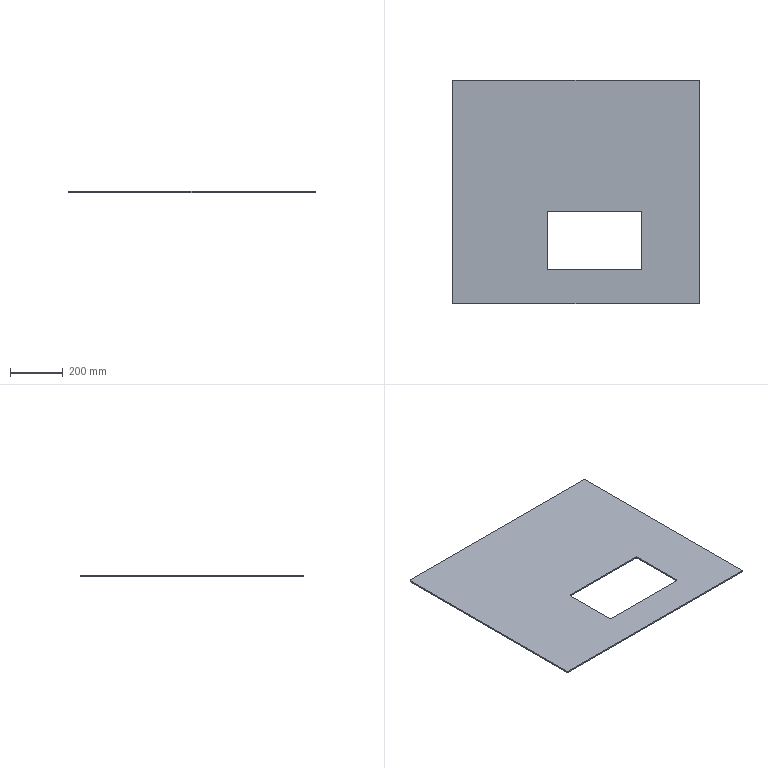Part | STEP file | 001-002-Face Plate-7 | 1 solid | 18 faces | box 940 x 850 x 5 mm | volume 3599000 mm3 | plane 10 | cylinder 8 | commonest cylinder face diameters 10 x8
STEP:
#1=CARTESIAN_POINT('',(0.,0.,0.));
#2=DIRECTION('',(0.,0.,1.));
#3=DIRECTION('',(1.,0.,0.));
#4=AXIS2_PLACEMENT_3D('',#1,#2,#3);
#5=CARTESIAN_POINT('',(470.,-420.,0.));
#6=VERTEX_POINT('',#5);
#7=CARTESIAN_POINT('',(470.,420.,0.));
#8=VERTEX_POINT('',#7);
#9=CARTESIAN_POINT('',(470.,-425.,0.));
#10=DIRECTION('',(0.,1.,0.));
#11=VECTOR('',#10,1.);
#12=LINE('',#9,#11);
#13=CARTESIAN_POINT('',(470.,-425.,5.));
#14=DIRECTION('',(-1.,0.,0.));
#15=DIRECTION('',(0.,0.,1.));
#16=AXIS2_PLACEMENT_3D('',#13,#14,#15);
#17=PLANE('',#16);
#18=CARTESIAN_POINT('',(-5.,0.));
#19=DIRECTION('',(0.,1.));
#20=VECTOR('',#19,1.);
#21=LINE('',#18,#20);
#22=(GEOMETRIC_REPRESENTATION_CONTEXT(2)PARAMETRIC_REPRESENTATION_CONTEXT()REPRESENTATION_CONTEXT('',''));
#23=DEFINITIONAL_REPRESENTATION('',(#21),#22);
#24=PCURVE('',#17,#23);
#25=CARTESIAN_POINT('',(0.,0.,0.));
#26=DIRECTION('',(0.,0.,-1.));
#27=DIRECTION('',(-1.,0.,0.));
#28=AXIS2_PLACEMENT_3D('',#25,#26,#27);
#29=PLANE('',#28);
#30=CARTESIAN_POINT('',(-470.,-425.));
#31=DIRECTION('',(0.,1.));
#32=VECTOR('',#31,1.);
#33=LINE('',#30,#32);
#34=(GEOMETRIC_REPRESENTATION_CONTEXT(2)PARAMETRIC_REPRESENTATION_CONTEXT()REPRESENTATION_CONTEXT('',''));
#35=DEFINITIONAL_REPRESENTATION('',(#33),#34);
#36=PCURVE('',#29,#35);
#37=SURFACE_CURVE('',#12,(#24,#36),.PCURVE_S1.);
#38=EDGE_CURVE('',#6,#8,#37,.T.);
#39=ORIENTED_EDGE('',*,*,#38,.T.);
#40=CARTESIAN_POINT('',(470.,420.,5.));
#41=VERTEX_POINT('',#40);
#42=CARTESIAN_POINT('',(470.,420.,5.));
#43=DIRECTION('',(0.,0.,1.));
#44=VECTOR('',#43,1.);
#45=LINE('',#42,#44);
#46=CARTESIAN_POINT('',(0.,845.));
#47=DIRECTION('',(1.,0.));
#48=VECTOR('',#47,1.);
#49=LINE('',#46,#48);
#50=(GEOMETRIC_REPRESENTATION_CONTEXT(2)PARAMETRIC_REPRESENTATION_CONTEXT()REPRESENTATION_CONTEXT('',''));
#51=DEFINITIONAL_REPRESENTATION('',(#49),#50);
#52=PCURVE('',#17,#51);
#53=CARTESIAN_POINT('',(465.,420.,5.));
#54=DIRECTION('',(0.,0.,-1.));
#55=DIRECTION('',(-1.,0.,0.));
#56=AXIS2_PLACEMENT_3D('',#53,#54,#55);
#57=CYLINDRICAL_SURFACE('',#56,5.);
#58=CARTESIAN_POINT('',(3.142,0.));
#59=DIRECTION('',(0.,-1.));
#60=VECTOR('',#59,1.);
#61=LINE('',#58,#60);
#62=(GEOMETRIC_REPRESENTATION_CONTEXT(2)PARAMETRIC_REPRESENTATION_CONTEXT()REPRESENTATION_CONTEXT('',''));
#63=DEFINITIONAL_REPRESENTATION('',(#61),#62);
#64=PCURVE('',#57,#63);
#65=SURFACE_CURVE('',#45,(#52,#64),.PCURVE_S1.);
#66=EDGE_CURVE('',#8,#41,#65,.T.);
#67=ORIENTED_EDGE('',*,*,#66,.T.);
#68=CARTESIAN_POINT('',(470.,-420.,5.));
#69=VERTEX_POINT('',#68);
#70=CARTESIAN_POINT('',(470.,-425.,5.));
#71=DIRECTION('',(0.,1.,0.));
#72=VECTOR('',#71,1.);
#73=LINE('',#70,#72);
#74=CARTESIAN_POINT('',(0.,0.));
#75=DIRECTION('',(0.,1.));
#76=VECTOR('',#75,1.);
#77=LINE('',#74,#76);
#78=(GEOMETRIC_REPRESENTATION_CONTEXT(2)PARAMETRIC_REPRESENTATION_CONTEXT()REPRESENTATION_CONTEXT('',''));
#79=DEFINITIONAL_REPRESENTATION('',(#77),#78);
#80=PCURVE('',#17,#79);
#81=CARTESIAN_POINT('',(0.,0.,5.));
#82=DIRECTION('',(0.,0.,-1.));
#83=DIRECTION('',(-1.,0.,0.));
#84=AXIS2_PLACEMENT_3D('',#81,#82,#83);
#85=PLANE('',#84);
#86=CARTESIAN_POINT('',(-470.,-425.));
#87=DIRECTION('',(0.,1.));
#88=VECTOR('',#87,1.);
#89=LINE('',#86,#88);
#90=(GEOMETRIC_REPRESENTATION_CONTEXT(2)PARAMETRIC_REPRESENTATION_CONTEXT()REPRESENTATION_CONTEXT('',''));
#91=DEFINITIONAL_REPRESENTATION('',(#89),#90);
#92=PCURVE('',#85,#91);
#93=SURFACE_CURVE('',#73,(#80,#92),.PCURVE_S1.);
#94=EDGE_CURVE('',#69,#41,#93,.T.);
#95=ORIENTED_EDGE('',*,*,#94,.F.);
#96=CARTESIAN_POINT('',(470.,-420.,5.));
#97=DIRECTION('',(0.,0.,-1.));
#98=VECTOR('',#97,1.);
#99=LINE('',#96,#98);
#100=CARTESIAN_POINT('',(0.,5.));
#101=DIRECTION('',(-1.,0.));
#102=VECTOR('',#101,1.);
#103=LINE('',#100,#102);
#104=(GEOMETRIC_REPRESENTATION_CONTEXT(2)PARAMETRIC_REPRESENTATION_CONTEXT()REPRESENTATION_CONTEXT('',''));
#105=DEFINITIONAL_REPRESENTATION('',(#103),#104);
#106=PCURVE('',#17,#105);
#107=CARTESIAN_POINT('',(465.,-420.,5.));
#108=DIRECTION('',(0.,0.,-1.));
#109=DIRECTION('',(-1.,0.,0.));
#110=AXIS2_PLACEMENT_3D('',#107,#108,#109);
#111=CYLINDRICAL_SURFACE('',#110,5.);
#112=CARTESIAN_POINT('',(3.142,0.));
#113=DIRECTION('',(0.,1.));
#114=VECTOR('',#113,1.);
#115=LINE('',#112,#114);
#116=(GEOMETRIC_REPRESENTATION_CONTEXT(2)PARAMETRIC_REPRESENTATION_CONTEXT()REPRESENTATION_CONTEXT('',''));
#117=DEFINITIONAL_REPRESENTATION('',(#115),#116);
#118=PCURVE('',#111,#117);
#119=SURFACE_CURVE('',#99,(#106,#118),.PCURVE_S1.);
#120=EDGE_CURVE('',#69,#6,#119,.T.);
#121=ORIENTED_EDGE('',*,*,#120,.T.);
#122=EDGE_LOOP('',(#39,#67,#95,#121));
#123=FACE_BOUND('',#122,.T.);
#124=ADVANCED_FACE('',(#123),#17,.F.);
#125=CARTESIAN_POINT('',(465.,425.,0.));
#126=VERTEX_POINT('',#125);
#127=CARTESIAN_POINT('',(-465.,425.,0.));
#128=VERTEX_POINT('',#127);
#129=CARTESIAN_POINT('',(-470.,425.,0.));
#130=DIRECTION('',(-1.,0.,0.));
#131=VECTOR('',#130,1.);
#132=LINE('',#129,#131);
#133=CARTESIAN_POINT('',(-470.,425.,5.));
#134=DIRECTION('',(0.,-1.,0.));
#135=DIRECTION('',(0.,0.,-1.));
#136=AXIS2_PLACEMENT_3D('',#133,#134,#135);
#137=PLANE('',#136);
#138=CARTESIAN_POINT('',(5.,0.));
#139=DIRECTION('',(0.,-1.));
#140=VECTOR('',#139,1.);
#141=LINE('',#138,#140);
#142=(GEOMETRIC_REPRESENTATION_CONTEXT(2)PARAMETRIC_REPRESENTATION_CONTEXT()REPRESENTATION_CONTEXT('',''));
#143=DEFINITIONAL_REPRESENTATION('',(#141),#142);
#144=PCURVE('',#137,#143);
#145=CARTESIAN_POINT('',(470.,425.));
#146=DIRECTION('',(1.,0.));
#147=VECTOR('',#146,1.);
#148=LINE('',#145,#147);
#149=(GEOMETRIC_REPRESENTATION_CONTEXT(2)PARAMETRIC_REPRESENTATION_CONTEXT()REPRESENTATION_CONTEXT('',''));
#150=DEFINITIONAL_REPRESENTATION('',(#148),#149);
#151=PCURVE('',#29,#150);
#152=SURFACE_CURVE('',#132,(#144,#151),.PCURVE_S1.);
#153=EDGE_CURVE('',#126,#128,#152,.T.);
#154=ORIENTED_EDGE('',*,*,#153,.T.);
#155=CARTESIAN_POINT('',(-465.,425.,5.));
#156=VERTEX_POINT('',#155);
#157=CARTESIAN_POINT('',(-465.,425.,5.));
#158=DIRECTION('',(0.,0.,1.));
#159=VECTOR('',#158,1.);
#160=LINE('',#157,#159);
#161=CARTESIAN_POINT('',(0.,5.));
#162=DIRECTION('',(-1.,0.));
#163=VECTOR('',#162,1.);
#164=LINE('',#161,#163);
#165=(GEOMETRIC_REPRESENTATION_CONTEXT(2)PARAMETRIC_REPRESENTATION_CONTEXT()REPRESENTATION_CONTEXT('',''));
#166=DEFINITIONAL_REPRESENTATION('',(#164),#165);
#167=PCURVE('',#137,#166);
#168=CARTESIAN_POINT('',(-465.,420.,5.));
#169=DIRECTION('',(0.,0.,-1.));
#170=DIRECTION('',(-1.,0.,0.));
#171=AXIS2_PLACEMENT_3D('',#168,#169,#170);
#172=CYLINDRICAL_SURFACE('',#171,5.);
#173=CARTESIAN_POINT('',(1.571,0.));
#174=DIRECTION('',(0.,-1.));
#175=VECTOR('',#174,1.);
#176=LINE('',#173,#175);
#177=(GEOMETRIC_REPRESENTATION_CONTEXT(2)PARAMETRIC_REPRESENTATION_CONTEXT()REPRESENTATION_CONTEXT('',''));
#178=DEFINITIONAL_REPRESENTATION('',(#176),#177);
#179=PCURVE('',#172,#178);
#180=SURFACE_CURVE('',#160,(#167,#179),.PCURVE_S1.);
#181=EDGE_CURVE('',#128,#156,#180,.T.);
#182=ORIENTED_EDGE('',*,*,#181,.T.);
#183=CARTESIAN_POINT('',(465.,425.,5.));
#184=VERTEX_POINT('',#183);
#185=CARTESIAN_POINT('',(-470.,425.,5.));
#186=DIRECTION('',(-1.,0.,0.));
#187=VECTOR('',#186,1.);
#188=LINE('',#185,#187);
#189=CARTESIAN_POINT('',(0.,0.));
#190=DIRECTION('',(0.,-1.));
#191=VECTOR('',#190,1.);
#192=LINE('',#189,#191);
#193=(GEOMETRIC_REPRESENTATION_CONTEXT(2)PARAMETRIC_REPRESENTATION_CONTEXT()REPRESENTATION_CONTEXT('',''));
#194=DEFINITIONAL_REPRESENTATION('',(#192),#193);
#195=PCURVE('',#137,#194);
#196=CARTESIAN_POINT('',(470.,425.));
#197=DIRECTION('',(1.,0.));
#198=VECTOR('',#197,1.);
#199=LINE('',#196,#198);
#200=(GEOMETRIC_REPRESENTATION_CONTEXT(2)PARAMETRIC_REPRESENTATION_CONTEXT()REPRESENTATION_CONTEXT('',''));
#201=DEFINITIONAL_REPRESENTATION('',(#199),#200);
#202=PCURVE('',#85,#201);
#203=SURFACE_CURVE('',#188,(#195,#202),.PCURVE_S1.);
#204=EDGE_CURVE('',#184,#156,#203,.T.);
#205=ORIENTED_EDGE('',*,*,#204,.F.);
#206=CARTESIAN_POINT('',(465.,425.,5.));
#207=DIRECTION('',(0.,0.,-1.));
#208=VECTOR('',#207,1.);
#209=LINE('',#206,#208);
#210=CARTESIAN_POINT('',(0.,935.));
#211=DIRECTION('',(1.,0.));
#212=VECTOR('',#211,1.);
#213=LINE('',#210,#212);
#214=(GEOMETRIC_REPRESENTATION_CONTEXT(2)PARAMETRIC_REPRESENTATION_CONTEXT()REPRESENTATION_CONTEXT('',''));
#215=DEFINITIONAL_REPRESENTATION('',(#213),#214);
#216=PCURVE('',#137,#215);
#217=CARTESIAN_POINT('',(1.571,0.));
#218=DIRECTION('',(0.,1.));
#219=VECTOR('',#218,1.);
#220=LINE('',#217,#219);
#221=(GEOMETRIC_REPRESENTATION_CONTEXT(2)PARAMETRIC_REPRESENTATION_CONTEXT()REPRESENTATION_CONTEXT('',''));
#222=DEFINITIONAL_REPRESENTATION('',(#220),#221);
#223=PCURVE('',#57,#222);
#224=SURFACE_CURVE('',#209,(#216,#223),.PCURVE_S1.);
#225=EDGE_CURVE('',#184,#126,#224,.T.);
#226=ORIENTED_EDGE('',*,*,#225,.T.);
#227=EDGE_LOOP('',(#154,#182,#205,#226));
#228=FACE_BOUND('',#227,.T.);
#229=ADVANCED_FACE('',(#228),#137,.F.);
#230=CARTESIAN_POINT('',(-470.,420.,0.));
#231=VERTEX_POINT('',#230);
#232=CARTESIAN_POINT('',(-470.,-420.,0.));
#233=VERTEX_POINT('',#232);
#234=CARTESIAN_POINT('',(-470.,-425.,0.));
#235=DIRECTION('',(0.,-1.,0.));
#236=VECTOR('',#235,1.);
#237=LINE('',#234,#236);
#238=CARTESIAN_POINT('',(-470.,-425.,5.));
#239=DIRECTION('',(1.,0.,0.));
#240=DIRECTION('',(0.,0.,-1.));
#241=AXIS2_PLACEMENT_3D('',#238,#239,#240);
#242=PLANE('',#241);
#243=CARTESIAN_POINT('',(5.,0.));
#244=DIRECTION('',(0.,-1.));
#245=VECTOR('',#244,1.);
#246=LINE('',#243,#245);
#247=(GEOMETRIC_REPRESENTATION_CONTEXT(2)PARAMETRIC_REPRESENTATION_CONTEXT()REPRESENTATION_CONTEXT('',''));
#248=DEFINITIONAL_REPRESENTATION('',(#246),#247);
#249=PCURVE('',#242,#248);
#250=CARTESIAN_POINT('',(470.,-425.));
#251=DIRECTION('',(0.,-1.));
#252=VECTOR('',#251,1.);
#253=LINE('',#250,#252);
#254=(GEOMETRIC_REPRESENTATION_CONTEXT(2)PARAMETRIC_REPRESENTATION_CONTEXT()REPRESENTATION_CONTEXT('',''));
#255=DEFINITIONAL_REPRESENTATION('',(#253),#254);
#256=PCURVE('',#29,#255);
#257=SURFACE_CURVE('',#237,(#249,#256),.PCURVE_S1.);
#258=EDGE_CURVE('',#231,#233,#257,.T.);
#259=ORIENTED_EDGE('',*,*,#258,.T.);
#260=CARTESIAN_POINT('',(-470.,-420.,5.));
#261=VERTEX_POINT('',#260);
#262=CARTESIAN_POINT('',(-470.,-420.,5.));
#263=DIRECTION('',(0.,0.,1.));
#264=VECTOR('',#263,1.);
#265=LINE('',#262,#264);
#266=CARTESIAN_POINT('',(0.,5.));
#267=DIRECTION('',(-1.,0.));
#268=VECTOR('',#267,1.);
#269=LINE('',#266,#268);
#270=(GEOMETRIC_REPRESENTATION_CONTEXT(2)PARAMETRIC_REPRESENTATION_CONTEXT()REPRESENTATION_CONTEXT('',''));
#271=DEFINITIONAL_REPRESENTATION('',(#269),#270);
#272=PCURVE('',#242,#271);
#273=CARTESIAN_POINT('',(-465.,-420.,5.));
#274=DIRECTION('',(0.,0.,-1.));
#275=DIRECTION('',(-1.,0.,0.));
#276=AXIS2_PLACEMENT_3D('',#273,#274,#275);
#277=CYLINDRICAL_SURFACE('',#276,5.);
#278=CARTESIAN_POINT('',(6.283,0.));
#279=DIRECTION('',(0.,-1.));
#280=VECTOR('',#279,1.);
#281=LINE('',#278,#280);
#282=(GEOMETRIC_REPRESENTATION_CONTEXT(2)PARAMETRIC_REPRESENTATION_CONTEXT()REPRESENTATION_CONTEXT('',''));
#283=DEFINITIONAL_REPRESENTATION('',(#281),#282);
#284=PCURVE('',#277,#283);
#285=SURFACE_CURVE('',#265,(#272,#284),.PCURVE_S1.);
#286=EDGE_CURVE('',#233,#261,#285,.T.);
#287=ORIENTED_EDGE('',*,*,#286,.T.);
#288=CARTESIAN_POINT('',(-470.,420.,5.));
#289=VERTEX_POINT('',#288);
#290=CARTESIAN_POINT('',(-470.,-425.,5.));
#291=DIRECTION('',(0.,-1.,0.));
#292=VECTOR('',#291,1.);
#293=LINE('',#290,#292);
#294=CARTESIAN_POINT('',(0.,0.));
#295=DIRECTION('',(0.,-1.));
#296=VECTOR('',#295,1.);
#297=LINE('',#294,#296);
#298=(GEOMETRIC_REPRESENTATION_CONTEXT(2)PARAMETRIC_REPRESENTATION_CONTEXT()REPRESENTATION_CONTEXT('',''));
#299=DEFINITIONAL_REPRESENTATION('',(#297),#298);
#300=PCURVE('',#242,#299);
#301=CARTESIAN_POINT('',(470.,-425.));
#302=DIRECTION('',(0.,-1.));
#303=VECTOR('',#302,1.);
#304=LINE('',#301,#303);
#305=(GEOMETRIC_REPRESENTATION_CONTEXT(2)PARAMETRIC_REPRESENTATION_CONTEXT()REPRESENTATION_CONTEXT('',''));
#306=DEFINITIONAL_REPRESENTATION('',(#304),#305);
#307=PCURVE('',#85,#306);
#308=SURFACE_CURVE('',#293,(#300,#307),.PCURVE_S1.);
#309=EDGE_CURVE('',#289,#261,#308,.T.);
#310=ORIENTED_EDGE('',*,*,#309,.F.);
#311=CARTESIAN_POINT('',(-470.,420.,5.));
#312=DIRECTION('',(0.,0.,-1.));
#313=VECTOR('',#312,1.);
#314=LINE('',#311,#313);
#315=CARTESIAN_POINT('',(0.,845.));
#316=DIRECTION('',(1.,0.));
#317=VECTOR('',#316,1.);
#318=LINE('',#315,#317);
#319=(GEOMETRIC_REPRESENTATION_CONTEXT(2)PARAMETRIC_REPRESENTATION_CONTEXT()REPRESENTATION_CONTEXT('',''));
#320=DEFINITIONAL_REPRESENTATION('',(#318),#319);
#321=PCURVE('',#242,#320);
#322=CARTESIAN_POINT('',(0.,0.));
#323=DIRECTION('',(0.,1.));
#324=VECTOR('',#323,1.);
#325=LINE('',#322,#324);
#326=(GEOMETRIC_REPRESENTATION_CONTEXT(2)PARAMETRIC_REPRESENTATION_CONTEXT()REPRESENTATION_CONTEXT('',''));
#327=DEFINITIONAL_REPRESENTATION('',(#325),#326);
#328=PCURVE('',#172,#327);
#329=SURFACE_CURVE('',#314,(#321,#328),.PCURVE_S1.);
#330=EDGE_CURVE('',#289,#231,#329,.T.);
#331=ORIENTED_EDGE('',*,*,#330,.T.);
#332=EDGE_LOOP('',(#259,#287,#310,#331));
#333=FACE_BOUND('',#332,.T.);
#334=ADVANCED_FACE('',(#333),#242,.F.);
#335=CARTESIAN_POINT('',(-465.,-425.,5.));
#336=VERTEX_POINT('',#335);
#337=CARTESIAN_POINT('',(465.,-425.,5.));
#338=VERTEX_POINT('',#337);
#339=CARTESIAN_POINT('',(-470.,-425.,5.));
#340=DIRECTION('',(1.,0.,0.));
#341=VECTOR('',#340,1.);
#342=LINE('',#339,#341);
#343=CARTESIAN_POINT('',(-470.,-425.,5.));
#344=DIRECTION('',(0.,1.,0.));
#345=DIRECTION('',(0.,0.,1.));
#346=AXIS2_PLACEMENT_3D('',#343,#344,#345);
#347=PLANE('',#346);
#348=CARTESIAN_POINT('',(0.,0.));
#349=DIRECTION('',(0.,1.));
#350=VECTOR('',#349,1.);
#351=LINE('',#348,#350);
#352=(GEOMETRIC_REPRESENTATION_CONTEXT(2)PARAMETRIC_REPRESENTATION_CONTEXT()REPRESENTATION_CONTEXT('',''));
#353=DEFINITIONAL_REPRESENTATION('',(#351),#352);
#354=PCURVE('',#347,#353);
#355=CARTESIAN_POINT('',(470.,-425.));
#356=DIRECTION('',(-1.,0.));
#357=VECTOR('',#356,1.);
#358=LINE('',#355,#357);
#359=(GEOMETRIC_REPRESENTATION_CONTEXT(2)PARAMETRIC_REPRESENTATION_CONTEXT()REPRESENTATION_CONTEXT('',''));
#360=DEFINITIONAL_REPRESENTATION('',(#358),#359);
#361=PCURVE('',#85,#360);
#362=SURFACE_CURVE('',#342,(#354,#361),.PCURVE_S1.);
#363=EDGE_CURVE('',#336,#338,#362,.T.);
#364=ORIENTED_EDGE('',*,*,#363,.F.);
#365=CARTESIAN_POINT('',(-465.,-425.,0.));
#366=VERTEX_POINT('',#365);
#367=CARTESIAN_POINT('',(-465.,-425.,5.));
#368=DIRECTION('',(0.,0.,-1.));
#369=VECTOR('',#368,1.);
#370=LINE('',#367,#369);
#371=CARTESIAN_POINT('',(0.,5.));
#372=DIRECTION('',(-1.,0.));
#373=VECTOR('',#372,1.);
#374=LINE('',#371,#373);
#375=(GEOMETRIC_REPRESENTATION_CONTEXT(2)PARAMETRIC_REPRESENTATION_CONTEXT()REPRESENTATION_CONTEXT('',''));
#376=DEFINITIONAL_REPRESENTATION('',(#374),#375);
#377=PCURVE('',#347,#376);
#378=CARTESIAN_POINT('',(4.712,0.));
#379=DIRECTION('',(0.,1.));
#380=VECTOR('',#379,1.);
#381=LINE('',#378,#380);
#382=(GEOMETRIC_REPRESENTATION_CONTEXT(2)PARAMETRIC_REPRESENTATION_CONTEXT()REPRESENTATION_CONTEXT('',''));
#383=DEFINITIONAL_REPRESENTATION('',(#381),#382);
#384=PCURVE('',#277,#383);
#385=SURFACE_CURVE('',#370,(#377,#384),.PCURVE_S1.);
#386=EDGE_CURVE('',#336,#366,#385,.T.);
#387=ORIENTED_EDGE('',*,*,#386,.T.);
#388=CARTESIAN_POINT('',(465.,-425.,0.));
#389=VERTEX_POINT('',#388);
#390=CARTESIAN_POINT('',(-470.,-425.,0.));
#391=DIRECTION('',(1.,0.,0.));
#392=VECTOR('',#391,1.);
#393=LINE('',#390,#392);
#394=CARTESIAN_POINT('',(-5.,0.));
#395=DIRECTION('',(0.,1.));
#396=VECTOR('',#395,1.);
#397=LINE('',#394,#396);
#398=(GEOMETRIC_REPRESENTATION_CONTEXT(2)PARAMETRIC_REPRESENTATION_CONTEXT()REPRESENTATION_CONTEXT('',''));
#399=DEFINITIONAL_REPRESENTATION('',(#397),#398);
#400=PCURVE('',#347,#399);
#401=CARTESIAN_POINT('',(470.,-425.));
#402=DIRECTION('',(-1.,0.));
#403=VECTOR('',#402,1.);
#404=LINE('',#401,#403);
#405=(GEOMETRIC_REPRESENTATION_CONTEXT(2)PARAMETRIC_REPRESENTATION_CONTEXT()REPRESENTATION_CONTEXT('',''));
#406=DEFINITIONAL_REPRESENTATION('',(#404),#405);
#407=PCURVE('',#29,#406);
#408=SURFACE_CURVE('',#393,(#400,#407),.PCURVE_S1.);
#409=EDGE_CURVE('',#366,#389,#408,.T.);
#410=ORIENTED_EDGE('',*,*,#409,.T.);
#411=CARTESIAN_POINT('',(465.,-425.,5.));
#412=DIRECTION('',(0.,0.,1.));
#413=VECTOR('',#412,1.);
#414=LINE('',#411,#413);
#415=CARTESIAN_POINT('',(0.,935.));
#416=DIRECTION('',(1.,0.));
#417=VECTOR('',#416,1.);
#418=LINE('',#415,#417);
#419=(GEOMETRIC_REPRESENTATION_CONTEXT(2)PARAMETRIC_REPRESENTATION_CONTEXT()REPRESENTATION_CONTEXT('',''));
#420=DEFINITIONAL_REPRESENTATION('',(#418),#419);
#421=PCURVE('',#347,#420);
#422=CARTESIAN_POINT('',(4.712,0.));
#423=DIRECTION('',(0.,-1.));
#424=VECTOR('',#423,1.);
#425=LINE('',#422,#424);
#426=(GEOMETRIC_REPRESENTATION_CONTEXT(2)PARAMETRIC_REPRESENTATION_CONTEXT()REPRESENTATION_CONTEXT('',''));
#427=DEFINITIONAL_REPRESENTATION('',(#425),#426);
#428=PCURVE('',#111,#427);
#429=SURFACE_CURVE('',#414,(#421,#428),.PCURVE_S1.);
#430=EDGE_CURVE('',#389,#338,#429,.T.);
#431=ORIENTED_EDGE('',*,*,#430,.T.);
#432=EDGE_LOOP('',(#364,#387,#410,#431));
#433=FACE_BOUND('',#432,.T.);
#434=ADVANCED_FACE('',(#433),#347,.F.);
#435=CARTESIAN_POINT('',(245.,-75.,5.));
#436=VERTEX_POINT('',#435);
#437=CARTESIAN_POINT('',(-105.,-75.,5.));
#438=VERTEX_POINT('',#437);
#439=CARTESIAN_POINT('',(250.,-75.,5.));
#440=DIRECTION('',(-1.,0.,0.));
#441=VECTOR('',#440,1.);
#442=LINE('',#439,#441);
#443=CARTESIAN_POINT('',(-250.,-75.));
#444=DIRECTION('',(1.,0.));
#445=VECTOR('',#444,1.);
#446=LINE('',#443,#445);
#447=(GEOMETRIC_REPRESENTATION_CONTEXT(2)PARAMETRIC_REPRESENTATION_CONTEXT()REPRESENTATION_CONTEXT('',''));
#448=DEFINITIONAL_REPRESENTATION('',(#446),#447);
#449=PCURVE('',#85,#448);
#450=CARTESIAN_POINT('',(250.,-75.,-5.));
#451=DIRECTION('',(0.,1.,0.));
#452=DIRECTION('',(-1.,0.,0.));
#453=AXIS2_PLACEMENT_3D('',#450,#451,#452);
#454=PLANE('',#453);
#455=CARTESIAN_POINT('',(0.,10.));
#456=DIRECTION('',(1.,0.));
#457=VECTOR('',#456,1.);
#458=LINE('',#455,#457);
#459=(GEOMETRIC_REPRESENTATION_CONTEXT(2)PARAMETRIC_REPRESENTATION_CONTEXT()REPRESENTATION_CONTEXT('',''));
#460=DEFINITIONAL_REPRESENTATION('',(#458),#459);
#461=PCURVE('',#454,#460);
#462=SURFACE_CURVE('',#442,(#449,#461),.PCURVE_S1.);
#463=EDGE_CURVE('',#436,#438,#462,.T.);
#464=ORIENTED_EDGE('',*,*,#463,.F.);
#465=CARTESIAN_POINT('',(250.,-80.,5.));
#466=VERTEX_POINT('',#465);
#467=CARTESIAN_POINT('',(245.,-80.,5.));
#468=DIRECTION('',(0.,0.,-1.));
#469=DIRECTION('',(-1.,0.,0.));
#470=AXIS2_PLACEMENT_3D('',#467,#468,#469);
#471=CIRCLE('',#470,5.);
#472=CARTESIAN_POINT('',(-245.,-80.));
#473=DIRECTION('',(1.,0.));
#474=AXIS2_PLACEMENT_2D('',#472,#473);
#475=CIRCLE('',#474,5.);
#476=(GEOMETRIC_REPRESENTATION_CONTEXT(2)PARAMETRIC_REPRESENTATION_CONTEXT()REPRESENTATION_CONTEXT('',''));
#477=DEFINITIONAL_REPRESENTATION('',(#475),#476);
#478=PCURVE('',#85,#477);
#479=CARTESIAN_POINT('',(245.,-80.,-5.));
#480=DIRECTION('',(0.,0.,-1.));
#481=DIRECTION('',(-1.,0.,0.));
#482=AXIS2_PLACEMENT_3D('',#479,#480,#481);
#483=CYLINDRICAL_SURFACE('',#482,5.);
#484=CARTESIAN_POINT('',(0.,-10.));
#485=DIRECTION('',(1.,0.));
#486=VECTOR('',#485,1.);
#487=LINE('',#484,#486);
#488=(GEOMETRIC_REPRESENTATION_CONTEXT(2)PARAMETRIC_REPRESENTATION_CONTEXT()REPRESENTATION_CONTEXT('',''));
#489=DEFINITIONAL_REPRESENTATION('',(#487),#488);
#490=PCURVE('',#483,#489);
#491=SURFACE_CURVE('',#471,(#478,#490),.PCURVE_S1.);
#492=EDGE_CURVE('',#436,#466,#491,.T.);
#493=ORIENTED_EDGE('',*,*,#492,.T.);
#494=CARTESIAN_POINT('',(250.,-290.,5.));
#495=VERTEX_POINT('',#494);
#496=CARTESIAN_POINT('',(250.,-295.,5.));
#497=DIRECTION('',(0.,1.,0.));
#498=VECTOR('',#497,1.);
#499=LINE('',#496,#498);
#500=CARTESIAN_POINT('',(-250.,-295.));
#501=DIRECTION('',(0.,1.));
#502=VECTOR('',#501,1.);
#503=LINE('',#500,#502);
#504=(GEOMETRIC_REPRESENTATION_CONTEXT(2)PARAMETRIC_REPRESENTATION_CONTEXT()REPRESENTATION_CONTEXT('',''));
#505=DEFINITIONAL_REPRESENTATION('',(#503),#504);
#506=PCURVE('',#85,#505);
#507=CARTESIAN_POINT('',(250.,-295.,-5.));
#508=DIRECTION('',(1.,0.,0.));
#509=DIRECTION('',(0.,0.,-1.));
#510=AXIS2_PLACEMENT_3D('',#507,#508,#509);
#511=PLANE('',#510);
#512=CARTESIAN_POINT('',(-10.,0.));
#513=DIRECTION('',(0.,1.));
#514=VECTOR('',#513,1.);
#515=LINE('',#512,#514);
#516=(GEOMETRIC_REPRESENTATION_CONTEXT(2)PARAMETRIC_REPRESENTATION_CONTEXT()REPRESENTATION_CONTEXT('',''));
#517=DEFINITIONAL_REPRESENTATION('',(#515),#516);
#518=PCURVE('',#511,#517);
#519=SURFACE_CURVE('',#499,(#506,#518),.PCURVE_S1.);
#520=EDGE_CURVE('',#495,#466,#519,.T.);
#521=ORIENTED_EDGE('',*,*,#520,.F.);
#522=CARTESIAN_POINT('',(245.,-295.,5.));
#523=VERTEX_POINT('',#522);
#524=CARTESIAN_POINT('',(245.,-290.,5.));
#525=DIRECTION('',(0.,0.,-1.));
#526=DIRECTION('',(-1.,0.,0.));
#527=AXIS2_PLACEMENT_3D('',#524,#525,#526);
#528=CIRCLE('',#527,5.);
#529=CARTESIAN_POINT('',(-245.,-290.));
#530=DIRECTION('',(1.,0.));
#531=AXIS2_PLACEMENT_2D('',#529,#530);
#532=CIRCLE('',#531,5.);
#533=(GEOMETRIC_REPRESENTATION_CONTEXT(2)PARAMETRIC_REPRESENTATION_CONTEXT()REPRESENTATION_CONTEXT('',''));
#534=DEFINITIONAL_REPRESENTATION('',(#532),#533);
#535=PCURVE('',#85,#534);
#536=CARTESIAN_POINT('',(245.,-290.,-5.));
#537=DIRECTION('',(0.,0.,-1.));
#538=DIRECTION('',(-1.,0.,0.));
#539=AXIS2_PLACEMENT_3D('',#536,#537,#538);
#540=CYLINDRICAL_SURFACE('',#539,5.);
#541=CARTESIAN_POINT('',(0.,-10.));
#542=DIRECTION('',(1.,0.));
#543=VECTOR('',#542,1.);
#544=LINE('',#541,#543);
#545=(GEOMETRIC_REPRESENTATION_CONTEXT(2)PARAMETRIC_REPRESENTATION_CONTEXT()REPRESENTATION_CONTEXT('',''));
#546=DEFINITIONAL_REPRESENTATION('',(#544),#545);
#547=PCURVE('',#540,#546);
#548=SURFACE_CURVE('',#528,(#535,#547),.PCURVE_S1.);
#549=EDGE_CURVE('',#495,#523,#548,.T.);
#550=ORIENTED_EDGE('',*,*,#549,.T.);
#551=CARTESIAN_POINT('',(-105.,-295.,5.));
#552=VERTEX_POINT('',#551);
#553=CARTESIAN_POINT('',(250.,-295.,5.));
#554=DIRECTION('',(1.,0.,0.));
#555=VECTOR('',#554,1.);
#556=LINE('',#553,#555);
#557=CARTESIAN_POINT('',(-250.,-295.));
#558=DIRECTION('',(-1.,0.));
#559=VECTOR('',#558,1.);
#560=LINE('',#557,#559);
#561=(GEOMETRIC_REPRESENTATION_CONTEXT(2)PARAMETRIC_REPRESENTATION_CONTEXT()REPRESENTATION_CONTEXT('',''));
#562=DEFINITIONAL_REPRESENTATION('',(#560),#561);
#563=PCURVE('',#85,#562);
#564=CARTESIAN_POINT('',(250.,-295.,-5.));
#565=DIRECTION('',(0.,-1.,0.));
#566=DIRECTION('',(1.,0.,0.));
#567=AXIS2_PLACEMENT_3D('',#564,#565,#566);
#568=PLANE('',#567);
#569=CARTESIAN_POINT('',(0.,10.));
#570=DIRECTION('',(1.,0.));
#571=VECTOR('',#570,1.);
#572=LINE('',#569,#571);
#573=(GEOMETRIC_REPRESENTATION_CONTEXT(2)PARAMETRIC_REPRESENTATION_CONTEXT()REPRESENTATION_CONTEXT('',''));
#574=DEFINITIONAL_REPRESENTATION('',(#572),#573);
#575=PCURVE('',#568,#574);
#576=SURFACE_CURVE('',#556,(#563,#575),.PCURVE_S1.);
#577=EDGE_CURVE('',#552,#523,#576,.T.);
#578=ORIENTED_EDGE('',*,*,#577,.F.);
#579=CARTESIAN_POINT('',(-110.,-290.,5.));
#580=VERTEX_POINT('',#579);
#581=CARTESIAN_POINT('',(-105.,-290.,5.));
#582=DIRECTION('',(0.,0.,-1.));
#583=DIRECTION('',(-1.,0.,0.));
#584=AXIS2_PLACEMENT_3D('',#581,#582,#583);
#585=CIRCLE('',#584,5.);
#586=CARTESIAN_POINT('',(105.,-290.));
#587=DIRECTION('',(1.,0.));
#588=AXIS2_PLACEMENT_2D('',#586,#587);
#589=CIRCLE('',#588,5.);
#590=(GEOMETRIC_REPRESENTATION_CONTEXT(2)PARAMETRIC_REPRESENTATION_CONTEXT()REPRESENTATION_CONTEXT('',''));
#591=DEFINITIONAL_REPRESENTATION('',(#589),#590);
#592=PCURVE('',#85,#591);
#593=CARTESIAN_POINT('',(-105.,-290.,-5.));
#594=DIRECTION('',(0.,0.,-1.));
#595=DIRECTION('',(-1.,0.,0.));
#596=AXIS2_PLACEMENT_3D('',#593,#594,#595);
#597=CYLINDRICAL_SURFACE('',#596,5.);
#598=CARTESIAN_POINT('',(0.,-10.));
#599=DIRECTION('',(1.,0.));
#600=VECTOR('',#599,1.);
#601=LINE('',#598,#600);
#602=(GEOMETRIC_REPRESENTATION_CONTEXT(2)PARAMETRIC_REPRESENTATION_CONTEXT()REPRESENTATION_CONTEXT('',''));
#603=DEFINITIONAL_REPRESENTATION('',(#601),#602);
#604=PCURVE('',#597,#603);
#605=SURFACE_CURVE('',#585,(#592,#604),.PCURVE_S1.);
#606=EDGE_CURVE('',#552,#580,#605,.T.);
#607=ORIENTED_EDGE('',*,*,#606,.T.);
#608=CARTESIAN_POINT('',(-110.,-80.,5.));
#609=VERTEX_POINT('',#608);
#610=CARTESIAN_POINT('',(-110.,-295.,5.));
#611=DIRECTION('',(0.,-1.,0.));
#612=VECTOR('',#611,1.);
#613=LINE('',#610,#612);
#614=CARTESIAN_POINT('',(110.,-295.));
#615=DIRECTION('',(0.,-1.));
#616=VECTOR('',#615,1.);
#617=LINE('',#614,#616);
#618=(GEOMETRIC_REPRESENTATION_CONTEXT(2)PARAMETRIC_REPRESENTATION_CONTEXT()REPRESENTATION_CONTEXT('',''));
#619=DEFINITIONAL_REPRESENTATION('',(#617),#618);
#620=PCURVE('',#85,#619);
#621=CARTESIAN_POINT('',(-110.,-295.,-5.));
#622=DIRECTION('',(-1.,0.,0.));
#623=DIRECTION('',(0.,0.,1.));
#624=AXIS2_PLACEMENT_3D('',#621,#622,#623);
#625=PLANE('',#624);
#626=CARTESIAN_POINT('',(10.,0.));
#627=DIRECTION('',(0.,-1.));
#628=VECTOR('',#627,1.);
#629=LINE('',#626,#628);
#630=(GEOMETRIC_REPRESENTATION_CONTEXT(2)PARAMETRIC_REPRESENTATION_CONTEXT()REPRESENTATION_CONTEXT('',''));
#631=DEFINITIONAL_REPRESENTATION('',(#629),#630);
#632=PCURVE('',#625,#631);
#633=SURFACE_CURVE('',#613,(#620,#632),.PCURVE_S1.);
#634=EDGE_CURVE('',#609,#580,#633,.T.);
#635=ORIENTED_EDGE('',*,*,#634,.F.);
#636=CARTESIAN_POINT('',(-105.,-80.,5.));
#637=DIRECTION('',(0.,0.,-1.));
#638=DIRECTION('',(-1.,0.,0.));
#639=AXIS2_PLACEMENT_3D('',#636,#637,#638);
#640=CIRCLE('',#639,5.);
#641=CARTESIAN_POINT('',(105.,-80.));
#642=DIRECTION('',(1.,0.));
#643=AXIS2_PLACEMENT_2D('',#641,#642);
#644=CIRCLE('',#643,5.);
#645=(GEOMETRIC_REPRESENTATION_CONTEXT(2)PARAMETRIC_REPRESENTATION_CONTEXT()REPRESENTATION_CONTEXT('',''));
#646=DEFINITIONAL_REPRESENTATION('',(#644),#645);
#647=PCURVE('',#85,#646);
#648=CARTESIAN_POINT('',(-105.,-80.,-5.));
#649=DIRECTION('',(0.,0.,-1.));
#650=DIRECTION('',(-1.,0.,0.));
#651=AXIS2_PLACEMENT_3D('',#648,#649,#650);
#652=CYLINDRICAL_SURFACE('',#651,5.);
#653=CARTESIAN_POINT('',(0.,-10.));
#654=DIRECTION('',(1.,0.));
#655=VECTOR('',#654,1.);
#656=LINE('',#653,#655);
#657=(GEOMETRIC_REPRESENTATION_CONTEXT(2)PARAMETRIC_REPRESENTATION_CONTEXT()REPRESENTATION_CONTEXT('',''));
#658=DEFINITIONAL_REPRESENTATION('',(#656),#657);
#659=PCURVE('',#652,#658);
#660=SURFACE_CURVE('',#640,(#647,#659),.PCURVE_S1.);
#661=EDGE_CURVE('',#609,#438,#660,.T.);
#662=ORIENTED_EDGE('',*,*,#661,.T.);
#663=EDGE_LOOP('',(#464,#493,#521,#550,#578,#607,#635,#662));
#664=FACE_BOUND('',#663,.T.);
#665=ORIENTED_EDGE('',*,*,#309,.T.);
#666=CARTESIAN_POINT('',(-465.,-420.,5.));
#667=DIRECTION('',(0.,0.,1.));
#668=DIRECTION('',(-1.,0.,0.));
#669=AXIS2_PLACEMENT_3D('',#666,#667,#668);
#670=CIRCLE('',#669,5.);
#671=CARTESIAN_POINT('',(470.,-420.));
#672=CARTESIAN_POINT('',(470.,-428.66));
#673=CARTESIAN_POINT('',(462.5,-424.33));
#674=CARTESIAN_POINT('',(455.,-420.));
#675=CARTESIAN_POINT('',(462.5,-415.67));
#676=CARTESIAN_POINT('',(470.,-411.34));
#677=CARTESIAN_POINT('',(470.,-420.));
#678=(BOUNDED_CURVE()B_SPLINE_CURVE(2,(#671,#672,#673,#674,#675,#676,#677),.UNSPECIFIED.,.T.,.F.)B_SPLINE_CURVE_WITH_KNOTS((1,2,2,2,2,1),(-2.094,0.,2.094,4.189,6.283,8.378),.UNSPECIFIED.)CURVE()GEOMETRIC_REPRESENTATION_ITEM()RATIONAL_B_SPLINE_CURVE((1.,0.5,1.,0.5,1.,0.5,1.))REPRESENTATION_ITEM(''));
#679=(GEOMETRIC_REPRESENTATION_CONTEXT(2)PARAMETRIC_REPRESENTATION_CONTEXT()REPRESENTATION_CONTEXT('',''));
#680=DEFINITIONAL_REPRESENTATION('',(#678),#679);
#681=PCURVE('',#85,#680);
#682=CARTESIAN_POINT('',(6.283,0.));
#683=DIRECTION('',(-1.,0.));
#684=VECTOR('',#683,1.);
#685=LINE('',#682,#684);
#686=(GEOMETRIC_REPRESENTATION_CONTEXT(2)PARAMETRIC_REPRESENTATION_CONTEXT()REPRESENTATION_CONTEXT('',''));
#687=DEFINITIONAL_REPRESENTATION('',(#685),#686);
#688=PCURVE('',#277,#687);
#689=SURFACE_CURVE('',#670,(#681,#688),.PCURVE_S1.);
#690=EDGE_CURVE('',#261,#336,#689,.T.);
#691=ORIENTED_EDGE('',*,*,#690,.T.);
#692=ORIENTED_EDGE('',*,*,#363,.T.);
#693=CARTESIAN_POINT('',(465.,-420.,5.));
#694=DIRECTION('',(0.,0.,1.));
#695=DIRECTION('',(-1.,0.,0.));
#696=AXIS2_PLACEMENT_3D('',#693,#694,#695);
#697=CIRCLE('',#696,5.);
#698=CARTESIAN_POINT('',(-460.,-420.));
#699=CARTESIAN_POINT('',(-460.,-428.66));
#700=CARTESIAN_POINT('',(-467.5,-424.33));
#701=CARTESIAN_POINT('',(-475.,-420.));
#702=CARTESIAN_POINT('',(-467.5,-415.67));
#703=CARTESIAN_POINT('',(-460.,-411.34));
#704=CARTESIAN_POINT('',(-460.,-420.));
#705=(BOUNDED_CURVE()B_SPLINE_CURVE(2,(#698,#699,#700,#701,#702,#703,#704),.UNSPECIFIED.,.T.,.F.)B_SPLINE_CURVE_WITH_KNOTS((1,2,2,2,2,1),(-2.094,0.,2.094,4.189,6.283,8.378),.UNSPECIFIED.)CURVE()GEOMETRIC_REPRESENTATION_ITEM()RATIONAL_B_SPLINE_CURVE((1.,0.5,1.,0.5,1.,0.5,1.))REPRESENTATION_ITEM(''));
#706=(GEOMETRIC_REPRESENTATION_CONTEXT(2)PARAMETRIC_REPRESENTATION_CONTEXT()REPRESENTATION_CONTEXT('',''));
#707=DEFINITIONAL_REPRESENTATION('',(#705),#706);
#708=PCURVE('',#85,#707);
#709=CARTESIAN_POINT('',(6.283,0.));
#710=DIRECTION('',(-1.,0.));
#711=VECTOR('',#710,1.);
#712=LINE('',#709,#711);
#713=(GEOMETRIC_REPRESENTATION_CONTEXT(2)PARAMETRIC_REPRESENTATION_CONTEXT()REPRESENTATION_CONTEXT('',''));
#714=DEFINITIONAL_REPRESENTATION('',(#712),#713);
#715=PCURVE('',#111,#714);
#716=SURFACE_CURVE('',#697,(#708,#715),.PCURVE_S1.);
#717=EDGE_CURVE('',#338,#69,#716,.T.);
#718=ORIENTED_EDGE('',*,*,#717,.T.);
#719=ORIENTED_EDGE('',*,*,#94,.T.);
#720=CARTESIAN_POINT('',(465.,420.,5.));
#721=DIRECTION('',(0.,0.,1.));
#722=DIRECTION('',(-1.,0.,0.));
#723=AXIS2_PLACEMENT_3D('',#720,#721,#722);
#724=CIRCLE('',#723,5.);
#725=CARTESIAN_POINT('',(-460.,420.));
#726=CARTESIAN_POINT('',(-460.,411.34));
#727=CARTESIAN_POINT('',(-467.5,415.67));
#728=CARTESIAN_POINT('',(-475.,420.));
#729=CARTESIAN_POINT('',(-467.5,424.33));
#730=CARTESIAN_POINT('',(-460.,428.66));
#731=CARTESIAN_POINT('',(-460.,420.));
#732=(BOUNDED_CURVE()B_SPLINE_CURVE(2,(#725,#726,#727,#728,#729,#730,#731),.UNSPECIFIED.,.T.,.F.)B_SPLINE_CURVE_WITH_KNOTS((1,2,2,2,2,1),(-2.094,0.,2.094,4.189,6.283,8.378),.UNSPECIFIED.)CURVE()GEOMETRIC_REPRESENTATION_ITEM()RATIONAL_B_SPLINE_CURVE((1.,0.5,1.,0.5,1.,0.5,1.))REPRESENTATION_ITEM(''));
#733=(GEOMETRIC_REPRESENTATION_CONTEXT(2)PARAMETRIC_REPRESENTATION_CONTEXT()REPRESENTATION_CONTEXT('',''));
#734=DEFINITIONAL_REPRESENTATION('',(#732),#733);
#735=PCURVE('',#85,#734);
#736=CARTESIAN_POINT('',(6.283,0.));
#737=DIRECTION('',(-1.,0.));
#738=VECTOR('',#737,1.);
#739=LINE('',#736,#738);
#740=(GEOMETRIC_REPRESENTATION_CONTEXT(2)PARAMETRIC_REPRESENTATION_CONTEXT()REPRESENTATION_CONTEXT('',''));
#741=DEFINITIONAL_REPRESENTATION('',(#739),#740);
#742=PCURVE('',#57,#741);
#743=SURFACE_CURVE('',#724,(#735,#742),.PCURVE_S1.);
#744=EDGE_CURVE('',#41,#184,#743,.T.);
#745=ORIENTED_EDGE('',*,*,#744,.T.);
#746=ORIENTED_EDGE('',*,*,#204,.T.);
#747=CARTESIAN_POINT('',(-465.,420.,5.));
#748=DIRECTION('',(0.,0.,1.));
#749=DIRECTION('',(-1.,0.,0.));
#750=AXIS2_PLACEMENT_3D('',#747,#748,#749);
#751=CIRCLE('',#750,5.);
#752=CARTESIAN_POINT('',(470.,420.));
#753=CARTESIAN_POINT('',(470.,411.34));
#754=CARTESIAN_POINT('',(462.5,415.67));
#755=CARTESIAN_POINT('',(455.,420.));
#756=CARTESIAN_POINT('',(462.5,424.33));
#757=CARTESIAN_POINT('',(470.,428.66));
#758=CARTESIAN_POINT('',(470.,420.));
#759=(BOUNDED_CURVE()B_SPLINE_CURVE(2,(#752,#753,#754,#755,#756,#757,#758),.UNSPECIFIED.,.T.,.F.)B_SPLINE_CURVE_WITH_KNOTS((1,2,2,2,2,1),(-2.094,0.,2.094,4.189,6.283,8.378),.UNSPECIFIED.)CURVE()GEOMETRIC_REPRESENTATION_ITEM()RATIONAL_B_SPLINE_CURVE((1.,0.5,1.,0.5,1.,0.5,1.))REPRESENTATION_ITEM(''));
#760=(GEOMETRIC_REPRESENTATION_CONTEXT(2)PARAMETRIC_REPRESENTATION_CONTEXT()REPRESENTATION_CONTEXT('',''));
#761=DEFINITIONAL_REPRESENTATION('',(#759),#760);
#762=PCURVE('',#85,#761);
#763=CARTESIAN_POINT('',(6.283,0.));
#764=DIRECTION('',(-1.,0.));
#765=VECTOR('',#764,1.);
#766=LINE('',#763,#765);
#767=(GEOMETRIC_REPRESENTATION_CONTEXT(2)PARAMETRIC_REPRESENTATION_CONTEXT()REPRESENTATION_CONTEXT('',''));
#768=DEFINITIONAL_REPRESENTATION('',(#766),#767);
#769=PCURVE('',#172,#768);
#770=SURFACE_CURVE('',#751,(#762,#769),.PCURVE_S1.);
#771=EDGE_CURVE('',#156,#289,#770,.T.);
#772=ORIENTED_EDGE('',*,*,#771,.T.);
#773=EDGE_LOOP('',(#665,#691,#692,#718,#719,#745,#746,#772));
#774=FACE_BOUND('',#773,.T.);
#775=ADVANCED_FACE('',(#664,#774),#85,.F.);
#776=CARTESIAN_POINT('',(250.,-80.,0.));
#777=VERTEX_POINT('',#776);
#778=CARTESIAN_POINT('',(250.,-290.,0.));
#779=VERTEX_POINT('',#778);
#780=CARTESIAN_POINT('',(250.,0.,0.));
#781=DIRECTION('',(0.,-1.,0.));
#782=VECTOR('',#781,1.);
#783=LINE('',#780,#782);
#784=CARTESIAN_POINT('',(-250.,0.));
#785=DIRECTION('',(0.,-1.));
#786=VECTOR('',#785,1.);
#787=LINE('',#784,#786);
#788=(GEOMETRIC_REPRESENTATION_CONTEXT(2)PARAMETRIC_REPRESENTATION_CONTEXT()REPRESENTATION_CONTEXT('',''));
#789=DEFINITIONAL_REPRESENTATION('',(#787),#788);
#790=PCURVE('',#29,#789);
#791=CARTESIAN_POINT('',(-5.,295.));
#792=DIRECTION('',(0.,-1.));
#793=VECTOR('',#792,1.);
#794=LINE('',#791,#793);
#795=(GEOMETRIC_REPRESENTATION_CONTEXT(2)PARAMETRIC_REPRESENTATION_CONTEXT()REPRESENTATION_CONTEXT('',''));
#796=DEFINITIONAL_REPRESENTATION('',(#794),#795);
#797=PCURVE('',#511,#796);
#798=SURFACE_CURVE('',#783,(#790,#797),.PCURVE_S1.);
#799=EDGE_CURVE('',#777,#779,#798,.T.);
#800=ORIENTED_EDGE('',*,*,#799,.F.);
#801=CARTESIAN_POINT('',(245.,-75.,0.));
#802=VERTEX_POINT('',#801);
#803=CARTESIAN_POINT('',(245.,-80.,0.));
#804=DIRECTION('',(0.,0.,1.));
#805=DIRECTION('',(-1.,0.,0.));
#806=AXIS2_PLACEMENT_3D('',#803,#804,#805);
#807=CIRCLE('',#806,5.);
#808=CARTESIAN_POINT('',(-240.,-80.));
#809=CARTESIAN_POINT('',(-240.,-88.66));
#810=CARTESIAN_POINT('',(-247.5,-84.33));
#811=CARTESIAN_POINT('',(-255.,-80.));
#812=CARTESIAN_POINT('',(-247.5,-75.67));
#813=CARTESIAN_POINT('',(-240.,-71.34));
#814=CARTESIAN_POINT('',(-240.,-80.));
#815=(BOUNDED_CURVE()B_SPLINE_CURVE(2,(#808,#809,#810,#811,#812,#813,#814),.UNSPECIFIED.,.T.,.F.)B_SPLINE_CURVE_WITH_KNOTS((1,2,2,2,2,1),(-2.094,0.,2.094,4.189,6.283,8.378),.UNSPECIFIED.)CURVE()GEOMETRIC_REPRESENTATION_ITEM()RATIONAL_B_SPLINE_CURVE((1.,0.5,1.,0.5,1.,0.5,1.))REPRESENTATION_ITEM(''));
#816=(GEOMETRIC_REPRESENTATION_CONTEXT(2)PARAMETRIC_REPRESENTATION_CONTEXT()REPRESENTATION_CONTEXT('',''));
#817=DEFINITIONAL_REPRESENTATION('',(#815),#816);
#818=PCURVE('',#29,#817);
#819=CARTESIAN_POINT('',(6.283,-5.));
#820=DIRECTION('',(-1.,0.));
#821=VECTOR('',#820,1.);
#822=LINE('',#819,#821);
#823=(GEOMETRIC_REPRESENTATION_CONTEXT(2)PARAMETRIC_REPRESENTATION_CONTEXT()REPRESENTATION_CONTEXT('',''));
#824=DEFINITIONAL_REPRESENTATION('',(#822),#823);
#825=PCURVE('',#483,#824);
#826=SURFACE_CURVE('',#807,(#818,#825),.PCURVE_S1.);
#827=EDGE_CURVE('',#777,#802,#826,.T.);
#828=ORIENTED_EDGE('',*,*,#827,.T.);
#829=CARTESIAN_POINT('',(-105.,-75.,0.));
#830=VERTEX_POINT('',#829);
#831=CARTESIAN_POINT('',(0.,-75.,0.));
#832=DIRECTION('',(1.,0.,0.));
#833=VECTOR('',#832,1.);
#834=LINE('',#831,#833);
#835=CARTESIAN_POINT('',(0.,-75.));
#836=DIRECTION('',(-1.,0.));
#837=VECTOR('',#836,1.);
#838=LINE('',#835,#837);
#839=(GEOMETRIC_REPRESENTATION_CONTEXT(2)PARAMETRIC_REPRESENTATION_CONTEXT()REPRESENTATION_CONTEXT('',''));
#840=DEFINITIONAL_REPRESENTATION('',(#838),#839);
#841=PCURVE('',#29,#840);
#842=CARTESIAN_POINT('',(250.,5.));
#843=DIRECTION('',(-1.,0.));
#844=VECTOR('',#843,1.);
#845=LINE('',#842,#844);
#846=(GEOMETRIC_REPRESENTATION_CONTEXT(2)PARAMETRIC_REPRESENTATION_CONTEXT()REPRESENTATION_CONTEXT('',''));
#847=DEFINITIONAL_REPRESENTATION('',(#845),#846);
#848=PCURVE('',#454,#847);
#849=SURFACE_CURVE('',#834,(#841,#848),.PCURVE_S1.);
#850=EDGE_CURVE('',#830,#802,#849,.T.);
#851=ORIENTED_EDGE('',*,*,#850,.F.);
#852=CARTESIAN_POINT('',(-110.,-80.,0.));
#853=VERTEX_POINT('',#852);
#854=CARTESIAN_POINT('',(-105.,-80.,0.));
#855=DIRECTION('',(0.,0.,1.));
#856=DIRECTION('',(-1.,0.,0.));
#857=AXIS2_PLACEMENT_3D('',#854,#855,#856);
#858=CIRCLE('',#857,5.);
#859=CARTESIAN_POINT('',(110.,-80.));
#860=CARTESIAN_POINT('',(110.,-88.66));
#861=CARTESIAN_POINT('',(102.5,-84.33));
#862=CARTESIAN_POINT('',(95.,-80.));
#863=CARTESIAN_POINT('',(102.5,-75.67));
#864=CARTESIAN_POINT('',(110.,-71.34));
#865=CARTESIAN_POINT('',(110.,-80.));
#866=(BOUNDED_CURVE()B_SPLINE_CURVE(2,(#859,#860,#861,#862,#863,#864,#865),.UNSPECIFIED.,.T.,.F.)B_SPLINE_CURVE_WITH_KNOTS((1,2,2,2,2,1),(-2.094,0.,2.094,4.189,6.283,8.378),.UNSPECIFIED.)CURVE()GEOMETRIC_REPRESENTATION_ITEM()RATIONAL_B_SPLINE_CURVE((1.,0.5,1.,0.5,1.,0.5,1.))REPRESENTATION_ITEM(''));
#867=(GEOMETRIC_REPRESENTATION_CONTEXT(2)PARAMETRIC_REPRESENTATION_CONTEXT()REPRESENTATION_CONTEXT('',''));
#868=DEFINITIONAL_REPRESENTATION('',(#866),#867);
#869=PCURVE('',#29,#868);
#870=CARTESIAN_POINT('',(6.283,-5.));
#871=DIRECTION('',(-1.,0.));
#872=VECTOR('',#871,1.);
#873=LINE('',#870,#872);
#874=(GEOMETRIC_REPRESENTATION_CONTEXT(2)PARAMETRIC_REPRESENTATION_CONTEXT()REPRESENTATION_CONTEXT('',''));
#875=DEFINITIONAL_REPRESENTATION('',(#873),#874);
#876=PCURVE('',#652,#875);
#877=SURFACE_CURVE('',#858,(#869,#876),.PCURVE_S1.);
#878=EDGE_CURVE('',#830,#853,#877,.T.);
#879=ORIENTED_EDGE('',*,*,#878,.T.);
#880=CARTESIAN_POINT('',(-110.,-290.,0.));
#881=VERTEX_POINT('',#880);
#882=CARTESIAN_POINT('',(-110.,0.,0.));
#883=DIRECTION('',(0.,1.,0.));
#884=VECTOR('',#883,1.);
#885=LINE('',#882,#884);
#886=CARTESIAN_POINT('',(110.,0.));
#887=DIRECTION('',(0.,1.));
#888=VECTOR('',#887,1.);
#889=LINE('',#886,#888);
#890=(GEOMETRIC_REPRESENTATION_CONTEXT(2)PARAMETRIC_REPRESENTATION_CONTEXT()REPRESENTATION_CONTEXT('',''));
#891=DEFINITIONAL_REPRESENTATION('',(#889),#890);
#892=PCURVE('',#29,#891);
#893=CARTESIAN_POINT('',(5.,295.));
#894=DIRECTION('',(0.,1.));
#895=VECTOR('',#894,1.);
#896=LINE('',#893,#895);
#897=(GEOMETRIC_REPRESENTATION_CONTEXT(2)PARAMETRIC_REPRESENTATION_CONTEXT()REPRESENTATION_CONTEXT('',''));
#898=DEFINITIONAL_REPRESENTATION('',(#896),#897);
#899=PCURVE('',#625,#898);
#900=SURFACE_CURVE('',#885,(#892,#899),.PCURVE_S1.);
#901=EDGE_CURVE('',#881,#853,#900,.T.);
#902=ORIENTED_EDGE('',*,*,#901,.F.);
#903=CARTESIAN_POINT('',(-105.,-295.,0.));
#904=VERTEX_POINT('',#903);
#905=CARTESIAN_POINT('',(-105.,-290.,0.));
#906=DIRECTION('',(0.,0.,1.));
#907=DIRECTION('',(-1.,0.,0.));
#908=AXIS2_PLACEMENT_3D('',#905,#906,#907);
#909=CIRCLE('',#908,5.);
#910=CARTESIAN_POINT('',(110.,-290.));
#911=CARTESIAN_POINT('',(110.,-298.66));
#912=CARTESIAN_POINT('',(102.5,-294.33));
#913=CARTESIAN_POINT('',(95.,-290.));
#914=CARTESIAN_POINT('',(102.5,-285.67));
#915=CARTESIAN_POINT('',(110.,-281.34));
#916=CARTESIAN_POINT('',(110.,-290.));
#917=(BOUNDED_CURVE()B_SPLINE_CURVE(2,(#910,#911,#912,#913,#914,#915,#916),.UNSPECIFIED.,.T.,.F.)B_SPLINE_CURVE_WITH_KNOTS((1,2,2,2,2,1),(-2.094,0.,2.094,4.189,6.283,8.378),.UNSPECIFIED.)CURVE()GEOMETRIC_REPRESENTATION_ITEM()RATIONAL_B_SPLINE_CURVE((1.,0.5,1.,0.5,1.,0.5,1.))REPRESENTATION_ITEM(''));
#918=(GEOMETRIC_REPRESENTATION_CONTEXT(2)PARAMETRIC_REPRESENTATION_CONTEXT()REPRESENTATION_CONTEXT('',''));
#919=DEFINITIONAL_REPRESENTATION('',(#917),#918);
#920=PCURVE('',#29,#919);
#921=CARTESIAN_POINT('',(6.283,-5.));
#922=DIRECTION('',(-1.,0.));
#923=VECTOR('',#922,1.);
#924=LINE('',#921,#923);
#925=(GEOMETRIC_REPRESENTATION_CONTEXT(2)PARAMETRIC_REPRESENTATION_CONTEXT()REPRESENTATION_CONTEXT('',''));
#926=DEFINITIONAL_REPRESENTATION('',(#924),#925);
#927=PCURVE('',#597,#926);
#928=SURFACE_CURVE('',#909,(#920,#927),.PCURVE_S1.);
#929=EDGE_CURVE('',#881,#904,#928,.T.);
#930=ORIENTED_EDGE('',*,*,#929,.T.);
#931=CARTESIAN_POINT('',(245.,-295.,0.));
#932=VERTEX_POINT('',#931);
#933=CARTESIAN_POINT('',(0.,-295.,0.));
#934=DIRECTION('',(-1.,0.,0.));
#935=VECTOR('',#934,1.);
#936=LINE('',#933,#935);
#937=CARTESIAN_POINT('',(0.,-295.));
#938=DIRECTION('',(1.,0.));
#939=VECTOR('',#938,1.);
#940=LINE('',#937,#939);
#941=(GEOMETRIC_REPRESENTATION_CONTEXT(2)PARAMETRIC_REPRESENTATION_CONTEXT()REPRESENTATION_CONTEXT('',''));
#942=DEFINITIONAL_REPRESENTATION('',(#940),#941);
#943=PCURVE('',#29,#942);
#944=CARTESIAN_POINT('',(-250.,5.));
#945=DIRECTION('',(-1.,0.));
#946=VECTOR('',#945,1.);
#947=LINE('',#944,#946);
#948=(GEOMETRIC_REPRESENTATION_CONTEXT(2)PARAMETRIC_REPRESENTATION_CONTEXT()REPRESENTATION_CONTEXT('',''));
#949=DEFINITIONAL_REPRESENTATION('',(#947),#948);
#950=PCURVE('',#568,#949);
#951=SURFACE_CURVE('',#936,(#943,#950),.PCURVE_S1.);
#952=EDGE_CURVE('',#932,#904,#951,.T.);
#953=ORIENTED_EDGE('',*,*,#952,.F.);
#954=CARTESIAN_POINT('',(245.,-290.,0.));
#955=DIRECTION('',(0.,0.,1.));
#956=DIRECTION('',(-1.,0.,0.));
#957=AXIS2_PLACEMENT_3D('',#954,#955,#956);
#958=CIRCLE('',#957,5.);
#959=CARTESIAN_POINT('',(-240.,-290.));
#960=CARTESIAN_POINT('',(-240.,-298.66));
#961=CARTESIAN_POINT('',(-247.5,-294.33));
#962=CARTESIAN_POINT('',(-255.,-290.));
#963=CARTESIAN_POINT('',(-247.5,-285.67));
#964=CARTESIAN_POINT('',(-240.,-281.34));
#965=CARTESIAN_POINT('',(-240.,-290.));
#966=(BOUNDED_CURVE()B_SPLINE_CURVE(2,(#959,#960,#961,#962,#963,#964,#965),.UNSPECIFIED.,.T.,.F.)B_SPLINE_CURVE_WITH_KNOTS((1,2,2,2,2,1),(-2.094,0.,2.094,4.189,6.283,8.378),.UNSPECIFIED.)CURVE()GEOMETRIC_REPRESENTATION_ITEM()RATIONAL_B_SPLINE_CURVE((1.,0.5,1.,0.5,1.,0.5,1.))REPRESENTATION_ITEM(''));
#967=(GEOMETRIC_REPRESENTATION_CONTEXT(2)PARAMETRIC_REPRESENTATION_CONTEXT()REPRESENTATION_CONTEXT('',''));
#968=DEFINITIONAL_REPRESENTATION('',(#966),#967);
#969=PCURVE('',#29,#968);
#970=CARTESIAN_POINT('',(6.283,-5.));
#971=DIRECTION('',(-1.,0.));
#972=VECTOR('',#971,1.);
#973=LINE('',#970,#972);
#974=(GEOMETRIC_REPRESENTATION_CONTEXT(2)PARAMETRIC_REPRESENTATION_CONTEXT()REPRESENTATION_CONTEXT('',''));
#975=DEFINITIONAL_REPRESENTATION('',(#973),#974);
#976=PCURVE('',#540,#975);
#977=SURFACE_CURVE('',#958,(#969,#976),.PCURVE_S1.);
#978=EDGE_CURVE('',#932,#779,#977,.T.);
#979=ORIENTED_EDGE('',*,*,#978,.T.);
#980=EDGE_LOOP('',(#800,#828,#851,#879,#902,#930,#953,#979));
#981=FACE_BOUND('',#980,.T.);
#982=ORIENTED_EDGE('',*,*,#409,.F.);
#983=CARTESIAN_POINT('',(-465.,-420.,0.));
#984=DIRECTION('',(0.,0.,-1.));
#985=DIRECTION('',(-1.,0.,0.));
#986=AXIS2_PLACEMENT_3D('',#983,#984,#985);
#987=CIRCLE('',#986,5.);
#988=CARTESIAN_POINT('',(465.,-420.));
#989=DIRECTION('',(1.,0.));
#990=AXIS2_PLACEMENT_2D('',#988,#989);
#991=CIRCLE('',#990,5.);
#992=(GEOMETRIC_REPRESENTATION_CONTEXT(2)PARAMETRIC_REPRESENTATION_CONTEXT()REPRESENTATION_CONTEXT('',''));
#993=DEFINITIONAL_REPRESENTATION('',(#991),#992);
#994=PCURVE('',#29,#993);
#995=CARTESIAN_POINT('',(0.,5.));
#996=DIRECTION('',(1.,0.));
#997=VECTOR('',#996,1.);
#998=LINE('',#995,#997);
#999=(GEOMETRIC_REPRESENTATION_CONTEXT(2)PARAMETRIC_REPRESENTATION_CONTEXT()REPRESENTATION_CONTEXT('',''));
#1000=DEFINITIONAL_REPRESENTATION('',(#998),#999);
#1001=PCURVE('',#277,#1000);
#1002=SURFACE_CURVE('',#987,(#994,#1001),.PCURVE_S1.);
#1003=EDGE_CURVE('',#366,#233,#1002,.T.);
#1004=ORIENTED_EDGE('',*,*,#1003,.T.);
#1005=ORIENTED_EDGE('',*,*,#258,.F.);
#1006=CARTESIAN_POINT('',(-465.,420.,0.));
#1007=DIRECTION('',(0.,0.,-1.));
#1008=DIRECTION('',(-1.,0.,0.));
#1009=AXIS2_PLACEMENT_3D('',#1006,#1007,#1008);
#1010=CIRCLE('',#1009,5.);
#1011=CARTESIAN_POINT('',(465.,420.));
#1012=DIRECTION('',(1.,0.));
#1013=AXIS2_PLACEMENT_2D('',#1011,#1012);
#1014=CIRCLE('',#1013,5.);
#1015=(GEOMETRIC_REPRESENTATION_CONTEXT(2)PARAMETRIC_REPRESENTATION_CONTEXT()REPRESENTATION_CONTEXT('',''));
#1016=DEFINITIONAL_REPRESENTATION('',(#1014),#1015);
#1017=PCURVE('',#29,#1016);
#1018=CARTESIAN_POINT('',(0.,5.));
#1019=DIRECTION('',(1.,0.));
#1020=VECTOR('',#1019,1.);
#1021=LINE('',#1018,#1020);
#1022=(GEOMETRIC_REPRESENTATION_CONTEXT(2)PARAMETRIC_REPRESENTATION_CONTEXT()REPRESENTATION_CONTEXT('',''));
#1023=DEFINITIONAL_REPRESENTATION('',(#1021),#1022);
#1024=PCURVE('',#172,#1023);
#1025=SURFACE_CURVE('',#1010,(#1017,#1024),.PCURVE_S1.);
#1026=EDGE_CURVE('',#231,#128,#1025,.T.);
#1027=ORIENTED_EDGE('',*,*,#1026,.T.);
#1028=ORIENTED_EDGE('',*,*,#153,.F.);
#1029=CARTESIAN_POINT('',(465.,420.,0.));
#1030=DIRECTION('',(0.,0.,-1.));
#1031=DIRECTION('',(-1.,0.,0.));
#1032=AXIS2_PLACEMENT_3D('',#1029,#1030,#1031);
#1033=CIRCLE('',#1032,5.);
#1034=CARTESIAN_POINT('',(-465.,420.));
#1035=DIRECTION('',(1.,0.));
#1036=AXIS2_PLACEMENT_2D('',#1034,#1035);
#1037=CIRCLE('',#1036,5.);
#1038=(GEOMETRIC_REPRESENTATION_CONTEXT(2)PARAMETRIC_REPRESENTATION_CONTEXT()REPRESENTATION_CONTEXT('',''));
#1039=DEFINITIONAL_REPRESENTATION('',(#1037),#1038);
#1040=PCURVE('',#29,#1039);
#1041=CARTESIAN_POINT('',(0.,5.));
#1042=DIRECTION('',(1.,0.));
#1043=VECTOR('',#1042,1.);
#1044=LINE('',#1041,#1043);
#1045=(GEOMETRIC_REPRESENTATION_CONTEXT(2)PARAMETRIC_REPRESENTATION_CONTEXT()REPRESENTATION_CONTEXT('',''));
#1046=DEFINITIONAL_REPRESENTATION('',(#1044),#1045);
#1047=PCURVE('',#57,#1046);
#1048=SURFACE_CURVE('',#1033,(#1040,#1047),.PCURVE_S1.);
#1049=EDGE_CURVE('',#126,#8,#1048,.T.);
#1050=ORIENTED_EDGE('',*,*,#1049,.T.);
#1051=ORIENTED_EDGE('',*,*,#38,.F.);
#1052=CARTESIAN_POINT('',(465.,-420.,0.));
#1053=DIRECTION('',(0.,0.,-1.));
#1054=DIRECTION('',(-1.,0.,0.));
#1055=AXIS2_PLACEMENT_3D('',#1052,#1053,#1054);
#1056=CIRCLE('',#1055,5.);
#1057=CARTESIAN_POINT('',(-465.,-420.));
#1058=DIRECTION('',(1.,0.));
#1059=AXIS2_PLACEMENT_2D('',#1057,#1058);
#1060=CIRCLE('',#1059,5.);
#1061=(GEOMETRIC_REPRESENTATION_CONTEXT(2)PARAMETRIC_REPRESENTATION_CONTEXT()REPRESENTATION_CONTEXT('',''));
#1062=DEFINITIONAL_REPRESENTATION('',(#1060),#1061);
#1063=PCURVE('',#29,#1062);
#1064=CARTESIAN_POINT('',(0.,5.));
#1065=DIRECTION('',(1.,0.));
#1066=VECTOR('',#1065,1.);
#1067=LINE('',#1064,#1066);
#1068=(GEOMETRIC_REPRESENTATION_CONTEXT(2)PARAMETRIC_REPRESENTATION_CONTEXT()REPRESENTATION_CONTEXT('',''));
#1069=DEFINITIONAL_REPRESENTATION('',(#1067),#1068);
#1070=PCURVE('',#111,#1069);
#1071=SURFACE_CURVE('',#1056,(#1063,#1070),.PCURVE_S1.);
#1072=EDGE_CURVE('',#6,#389,#1071,.T.);
#1073=ORIENTED_EDGE('',*,*,#1072,.T.);
#1074=EDGE_LOOP('',(#982,#1004,#1005,#1027,#1028,#1050,#1051,#1073));
#1075=FACE_BOUND('',#1074,.T.);
#1076=ADVANCED_FACE('',(#981,#1075),#29,.T.);
#1077=ORIENTED_EDGE('',*,*,#690,.F.);
#1078=ORIENTED_EDGE('',*,*,#286,.F.);
#1079=ORIENTED_EDGE('',*,*,#1003,.F.);
#1080=ORIENTED_EDGE('',*,*,#386,.F.);
#1081=EDGE_LOOP('',(#1077,#1078,#1079,#1080));
#1082=FACE_BOUND('',#1081,.T.);
#1083=ADVANCED_FACE('',(#1082),#277,.T.);
#1084=ORIENTED_EDGE('',*,*,#771,.F.);
#1085=ORIENTED_EDGE('',*,*,#181,.F.);
#1086=ORIENTED_EDGE('',*,*,#1026,.F.);
#1087=ORIENTED_EDGE('',*,*,#330,.F.);
#1088=EDGE_LOOP('',(#1084,#1085,#1086,#1087));
#1089=FACE_BOUND('',#1088,.T.);
#1090=ADVANCED_FACE('',(#1089),#172,.T.);
#1091=ORIENTED_EDGE('',*,*,#744,.F.);
#1092=ORIENTED_EDGE('',*,*,#66,.F.);
#1093=ORIENTED_EDGE('',*,*,#1049,.F.);
#1094=ORIENTED_EDGE('',*,*,#225,.F.);
#1095=EDGE_LOOP('',(#1091,#1092,#1093,#1094));
#1096=FACE_BOUND('',#1095,.T.);
#1097=ADVANCED_FACE('',(#1096),#57,.T.);
#1098=ORIENTED_EDGE('',*,*,#717,.F.);
#1099=ORIENTED_EDGE('',*,*,#430,.F.);
#1100=ORIENTED_EDGE('',*,*,#1072,.F.);
#1101=ORIENTED_EDGE('',*,*,#120,.F.);
#1102=EDGE_LOOP('',(#1098,#1099,#1100,#1101));
#1103=FACE_BOUND('',#1102,.T.);
#1104=ADVANCED_FACE('',(#1103),#111,.T.);
#1105=ORIENTED_EDGE('',*,*,#520,.T.);
#1106=CARTESIAN_POINT('',(250.,-80.,0.));
#1107=DIRECTION('',(0.,0.,-1.));
#1108=VECTOR('',#1107,1.);
#1109=LINE('',#1106,#1108);
#1110=CARTESIAN_POINT('',(-5.,215.));
#1111=DIRECTION('',(1.,0.));
#1112=VECTOR('',#1111,1.);
#1113=LINE('',#1110,#1112);
#1114=(GEOMETRIC_REPRESENTATION_CONTEXT(2)PARAMETRIC_REPRESENTATION_CONTEXT()REPRESENTATION_CONTEXT('',''));
#1115=DEFINITIONAL_REPRESENTATION('',(#1113),#1114);
#1116=PCURVE('',#511,#1115);
#1117=CARTESIAN_POINT('',(3.142,-5.));
#1118=DIRECTION('',(0.,1.));
#1119=VECTOR('',#1118,1.);
#1120=LINE('',#1117,#1119);
#1121=(GEOMETRIC_REPRESENTATION_CONTEXT(2)PARAMETRIC_REPRESENTATION_CONTEXT()REPRESENTATION_CONTEXT('',''));
#1122=DEFINITIONAL_REPRESENTATION('',(#1120),#1121);
#1123=PCURVE('',#483,#1122);
#1124=SURFACE_CURVE('',#1109,(#1116,#1123),.PCURVE_S1.);
#1125=EDGE_CURVE('',#466,#777,#1124,.T.);
#1126=ORIENTED_EDGE('',*,*,#1125,.T.);
#1127=ORIENTED_EDGE('',*,*,#799,.T.);
#1128=CARTESIAN_POINT('',(250.,-290.,5.));
#1129=DIRECTION('',(0.,0.,1.));
#1130=VECTOR('',#1129,1.);
#1131=LINE('',#1128,#1130);
#1132=CARTESIAN_POINT('',(-10.,5.));
#1133=DIRECTION('',(-1.,0.));
#1134=VECTOR('',#1133,1.);
#1135=LINE('',#1132,#1134);
#1136=(GEOMETRIC_REPRESENTATION_CONTEXT(2)PARAMETRIC_REPRESENTATION_CONTEXT()REPRESENTATION_CONTEXT('',''));
#1137=DEFINITIONAL_REPRESENTATION('',(#1135),#1136);
#1138=PCURVE('',#511,#1137);
#1139=CARTESIAN_POINT('',(3.142,-10.));
#1140=DIRECTION('',(0.,-1.));
#1141=VECTOR('',#1140,1.);
#1142=LINE('',#1139,#1141);
#1143=(GEOMETRIC_REPRESENTATION_CONTEXT(2)PARAMETRIC_REPRESENTATION_CONTEXT()REPRESENTATION_CONTEXT('',''));
#1144=DEFINITIONAL_REPRESENTATION('',(#1142),#1143);
#1145=PCURVE('',#540,#1144);
#1146=SURFACE_CURVE('',#1131,(#1138,#1145),.PCURVE_S1.);
#1147=EDGE_CURVE('',#779,#495,#1146,.T.);
#1148=ORIENTED_EDGE('',*,*,#1147,.T.);
#1149=EDGE_LOOP('',(#1105,#1126,#1127,#1148));
#1150=FACE_BOUND('',#1149,.T.);
#1151=ADVANCED_FACE('',(#1150),#511,.F.);
#1152=ORIENTED_EDGE('',*,*,#952,.T.);
#1153=CARTESIAN_POINT('',(-105.,-295.,5.));
#1154=DIRECTION('',(0.,0.,1.));
#1155=VECTOR('',#1154,1.);
#1156=LINE('',#1153,#1155);
#1157=CARTESIAN_POINT('',(-355.,10.));
#1158=DIRECTION('',(0.,1.));
#1159=VECTOR('',#1158,1.);
#1160=LINE('',#1157,#1159);
#1161=(GEOMETRIC_REPRESENTATION_CONTEXT(2)PARAMETRIC_REPRESENTATION_CONTEXT()REPRESENTATION_CONTEXT('',''));
#1162=DEFINITIONAL_REPRESENTATION('',(#1160),#1161);
#1163=PCURVE('',#568,#1162);
#1164=CARTESIAN_POINT('',(4.712,-10.));
#1165=DIRECTION('',(0.,-1.));
#1166=VECTOR('',#1165,1.);
#1167=LINE('',#1164,#1166);
#1168=(GEOMETRIC_REPRESENTATION_CONTEXT(2)PARAMETRIC_REPRESENTATION_CONTEXT()REPRESENTATION_CONTEXT('',''));
#1169=DEFINITIONAL_REPRESENTATION('',(#1167),#1168);
#1170=PCURVE('',#597,#1169);
#1171=SURFACE_CURVE('',#1156,(#1163,#1170),.PCURVE_S1.);
#1172=EDGE_CURVE('',#904,#552,#1171,.T.);
#1173=ORIENTED_EDGE('',*,*,#1172,.T.);
#1174=ORIENTED_EDGE('',*,*,#577,.T.);
#1175=CARTESIAN_POINT('',(245.,-295.,0.));
#1176=DIRECTION('',(0.,0.,-1.));
#1177=VECTOR('',#1176,1.);
#1178=LINE('',#1175,#1177);
#1179=CARTESIAN_POINT('',(-5.,5.));
#1180=DIRECTION('',(0.,-1.));
#1181=VECTOR('',#1180,1.);
#1182=LINE('',#1179,#1181);
#1183=(GEOMETRIC_REPRESENTATION_CONTEXT(2)PARAMETRIC_REPRESENTATION_CONTEXT()REPRESENTATION_CONTEXT('',''));
#1184=DEFINITIONAL_REPRESENTATION('',(#1182),#1183);
#1185=PCURVE('',#568,#1184);
#1186=CARTESIAN_POINT('',(4.712,-5.));
#1187=DIRECTION('',(0.,1.));
#1188=VECTOR('',#1187,1.);
#1189=LINE('',#1186,#1188);
#1190=(GEOMETRIC_REPRESENTATION_CONTEXT(2)PARAMETRIC_REPRESENTATION_CONTEXT()REPRESENTATION_CONTEXT('',''));
#1191=DEFINITIONAL_REPRESENTATION('',(#1189),#1190);
#1192=PCURVE('',#540,#1191);
#1193=SURFACE_CURVE('',#1178,(#1185,#1192),.PCURVE_S1.);
#1194=EDGE_CURVE('',#523,#932,#1193,.T.);
#1195=ORIENTED_EDGE('',*,*,#1194,.T.);
#1196=EDGE_LOOP('',(#1152,#1173,#1174,#1195));
#1197=FACE_BOUND('',#1196,.T.);
#1198=ADVANCED_FACE('',(#1197),#568,.F.);
#1199=ORIENTED_EDGE('',*,*,#634,.T.);
#1200=CARTESIAN_POINT('',(-110.,-290.,0.));
#1201=DIRECTION('',(0.,0.,-1.));
#1202=VECTOR('',#1201,1.);
#1203=LINE('',#1200,#1202);
#1204=CARTESIAN_POINT('',(5.,5.));
#1205=DIRECTION('',(-1.,0.));
#1206=VECTOR('',#1205,1.);
#1207=LINE('',#1204,#1206);
#1208=(GEOMETRIC_REPRESENTATION_CONTEXT(2)PARAMETRIC_REPRESENTATION_CONTEXT()REPRESENTATION_CONTEXT('',''));
#1209=DEFINITIONAL_REPRESENTATION('',(#1207),#1208);
#1210=PCURVE('',#625,#1209);
#1211=CARTESIAN_POINT('',(6.283,-5.));
#1212=DIRECTION('',(0.,1.));
#1213=VECTOR('',#1212,1.);
#1214=LINE('',#1211,#1213);
#1215=(GEOMETRIC_REPRESENTATION_CONTEXT(2)PARAMETRIC_REPRESENTATION_CONTEXT()REPRESENTATION_CONTEXT('',''));
#1216=DEFINITIONAL_REPRESENTATION('',(#1214),#1215);
#1217=PCURVE('',#597,#1216);
#1218=SURFACE_CURVE('',#1203,(#1210,#1217),.PCURVE_S1.);
#1219=EDGE_CURVE('',#580,#881,#1218,.T.);
#1220=ORIENTED_EDGE('',*,*,#1219,.T.);
#1221=ORIENTED_EDGE('',*,*,#901,.T.);
#1222=CARTESIAN_POINT('',(-110.,-80.,5.));
#1223=DIRECTION('',(0.,0.,1.));
#1224=VECTOR('',#1223,1.);
#1225=LINE('',#1222,#1224);
#1226=CARTESIAN_POINT('',(10.,215.));
#1227=DIRECTION('',(1.,0.));
#1228=VECTOR('',#1227,1.);
#1229=LINE('',#1226,#1228);
#1230=(GEOMETRIC_REPRESENTATION_CONTEXT(2)PARAMETRIC_REPRESENTATION_CONTEXT()REPRESENTATION_CONTEXT('',''));
#1231=DEFINITIONAL_REPRESENTATION('',(#1229),#1230);
#1232=PCURVE('',#625,#1231);
#1233=CARTESIAN_POINT('',(0.,-10.));
#1234=DIRECTION('',(0.,-1.));
#1235=VECTOR('',#1234,1.);
#1236=LINE('',#1233,#1235);
#1237=(GEOMETRIC_REPRESENTATION_CONTEXT(2)PARAMETRIC_REPRESENTATION_CONTEXT()REPRESENTATION_CONTEXT('',''));
#1238=DEFINITIONAL_REPRESENTATION('',(#1236),#1237);
#1239=PCURVE('',#652,#1238);
#1240=SURFACE_CURVE('',#1225,(#1232,#1239),.PCURVE_S1.);
#1241=EDGE_CURVE('',#853,#609,#1240,.T.);
#1242=ORIENTED_EDGE('',*,*,#1241,.T.);
#1243=EDGE_LOOP('',(#1199,#1220,#1221,#1242));
#1244=FACE_BOUND('',#1243,.T.);
#1245=ADVANCED_FACE('',(#1244),#625,.F.);
#1246=ORIENTED_EDGE('',*,*,#463,.T.);
#1247=CARTESIAN_POINT('',(-105.,-75.,0.));
#1248=DIRECTION('',(0.,0.,-1.));
#1249=VECTOR('',#1248,1.);
#1250=LINE('',#1247,#1249);
#1251=CARTESIAN_POINT('',(355.,5.));
#1252=DIRECTION('',(0.,-1.));
#1253=VECTOR('',#1252,1.);
#1254=LINE('',#1251,#1253);
#1255=(GEOMETRIC_REPRESENTATION_CONTEXT(2)PARAMETRIC_REPRESENTATION_CONTEXT()REPRESENTATION_CONTEXT('',''));
#1256=DEFINITIONAL_REPRESENTATION('',(#1254),#1255);
#1257=PCURVE('',#454,#1256);
#1258=CARTESIAN_POINT('',(1.571,-5.));
#1259=DIRECTION('',(0.,1.));
#1260=VECTOR('',#1259,1.);
#1261=LINE('',#1258,#1260);
#1262=(GEOMETRIC_REPRESENTATION_CONTEXT(2)PARAMETRIC_REPRESENTATION_CONTEXT()REPRESENTATION_CONTEXT('',''));
#1263=DEFINITIONAL_REPRESENTATION('',(#1261),#1262);
#1264=PCURVE('',#652,#1263);
#1265=SURFACE_CURVE('',#1250,(#1257,#1264),.PCURVE_S1.);
#1266=EDGE_CURVE('',#438,#830,#1265,.T.);
#1267=ORIENTED_EDGE('',*,*,#1266,.T.);
#1268=ORIENTED_EDGE('',*,*,#850,.T.);
#1269=CARTESIAN_POINT('',(245.,-75.,5.));
#1270=DIRECTION('',(0.,0.,1.));
#1271=VECTOR('',#1270,1.);
#1272=LINE('',#1269,#1271);
#1273=CARTESIAN_POINT('',(5.,10.));
#1274=DIRECTION('',(0.,1.));
#1275=VECTOR('',#1274,1.);
#1276=LINE('',#1273,#1275);
#1277=(GEOMETRIC_REPRESENTATION_CONTEXT(2)PARAMETRIC_REPRESENTATION_CONTEXT()REPRESENTATION_CONTEXT('',''));
#1278=DEFINITIONAL_REPRESENTATION('',(#1276),#1277);
#1279=PCURVE('',#454,#1278);
#1280=CARTESIAN_POINT('',(1.571,-10.));
#1281=DIRECTION('',(0.,-1.));
#1282=VECTOR('',#1281,1.);
#1283=LINE('',#1280,#1282);
#1284=(GEOMETRIC_REPRESENTATION_CONTEXT(2)PARAMETRIC_REPRESENTATION_CONTEXT()REPRESENTATION_CONTEXT('',''));
#1285=DEFINITIONAL_REPRESENTATION('',(#1283),#1284);
#1286=PCURVE('',#483,#1285);
#1287=SURFACE_CURVE('',#1272,(#1279,#1286),.PCURVE_S1.);
#1288=EDGE_CURVE('',#802,#436,#1287,.T.);
#1289=ORIENTED_EDGE('',*,*,#1288,.T.);
#1290=EDGE_LOOP('',(#1246,#1267,#1268,#1289));
#1291=FACE_BOUND('',#1290,.T.);
#1292=ADVANCED_FACE('',(#1291),#454,.F.);
#1293=ORIENTED_EDGE('',*,*,#1172,.T.);
#1294=ORIENTED_EDGE('',*,*,#606,.T.);
#1295=ORIENTED_EDGE('',*,*,#1219,.T.);
#1296=ORIENTED_EDGE('',*,*,#929,.T.);
#1297=EDGE_LOOP('',(#1293,#1294,#1295,#1296));
#1298=FACE_BOUND('',#1297,.F.);
#1299=ADVANCED_FACE('',(#1298),#597,.F.);
#1300=ORIENTED_EDGE('',*,*,#1241,.T.);
#1301=ORIENTED_EDGE('',*,*,#661,.T.);
#1302=ORIENTED_EDGE('',*,*,#1266,.T.);
#1303=ORIENTED_EDGE('',*,*,#878,.T.);
#1304=EDGE_LOOP('',(#1300,#1301,#1302,#1303));
#1305=FACE_BOUND('',#1304,.F.);
#1306=ADVANCED_FACE('',(#1305),#652,.F.);
#1307=ORIENTED_EDGE('',*,*,#1288,.T.);
#1308=ORIENTED_EDGE('',*,*,#492,.T.);
#1309=ORIENTED_EDGE('',*,*,#1125,.T.);
#1310=ORIENTED_EDGE('',*,*,#827,.T.);
#1311=EDGE_LOOP('',(#1307,#1308,#1309,#1310));
#1312=FACE_BOUND('',#1311,.F.);
#1313=ADVANCED_FACE('',(#1312),#483,.F.);
#1314=ORIENTED_EDGE('',*,*,#1147,.T.);
#1315=ORIENTED_EDGE('',*,*,#549,.T.);
#1316=ORIENTED_EDGE('',*,*,#1194,.T.);
#1317=ORIENTED_EDGE('',*,*,#978,.T.);
#1318=EDGE_LOOP('',(#1314,#1315,#1316,#1317));
#1319=FACE_BOUND('',#1318,.F.);
#1320=ADVANCED_FACE('',(#1319),#540,.F.);
#1321=CLOSED_SHELL('',(#124,#229,#334,#434,#775,#1076,#1083,#1090,#1097,#1104,#1151,#1198,#1245,#1292,#1299,#1306,#1313,#1320));
#1322=MANIFOLD_SOLID_BREP('',#1321);
#1323=(LENGTH_UNIT()NAMED_UNIT(*)SI_UNIT(.MILLI.,.METRE.));
#1324=UNCERTAINTY_MEASURE_WITH_UNIT(LENGTH_MEASURE(0.0000001),#1323,'','');
#1325=(NAMED_UNIT(*)PLANE_ANGLE_UNIT()SI_UNIT($,.RADIAN.));
#1326=(NAMED_UNIT(*)SI_UNIT($,.STERADIAN.)SOLID_ANGLE_UNIT());
#1327=(GEOMETRIC_REPRESENTATION_CONTEXT(3)GLOBAL_UNCERTAINTY_ASSIGNED_CONTEXT((#1324))GLOBAL_UNIT_ASSIGNED_CONTEXT((#1323,#1325,#1326))REPRESENTATION_CONTEXT('',''));
#1328=ADVANCED_BREP_SHAPE_REPRESENTATION('',(#4,#1322),#1327);